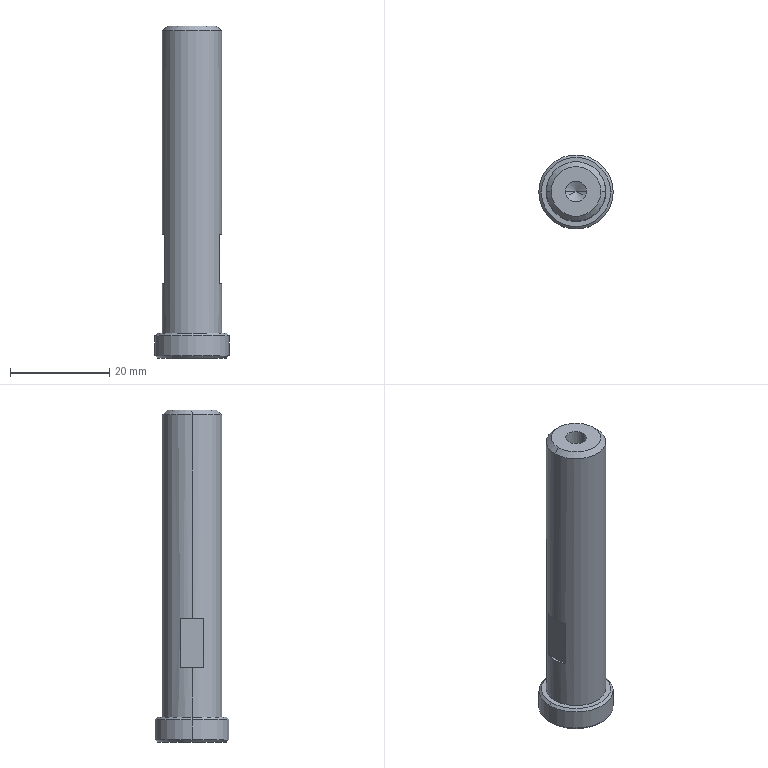Part | STEP file | 1 solid | 27 faces | box 15 x 15 x 67 mm | volume 7479 mm3 | cone 10 | plane 9 | cylinder 8 | commonest cylinder face diameters 4.2 x4 12 x2 15 x2